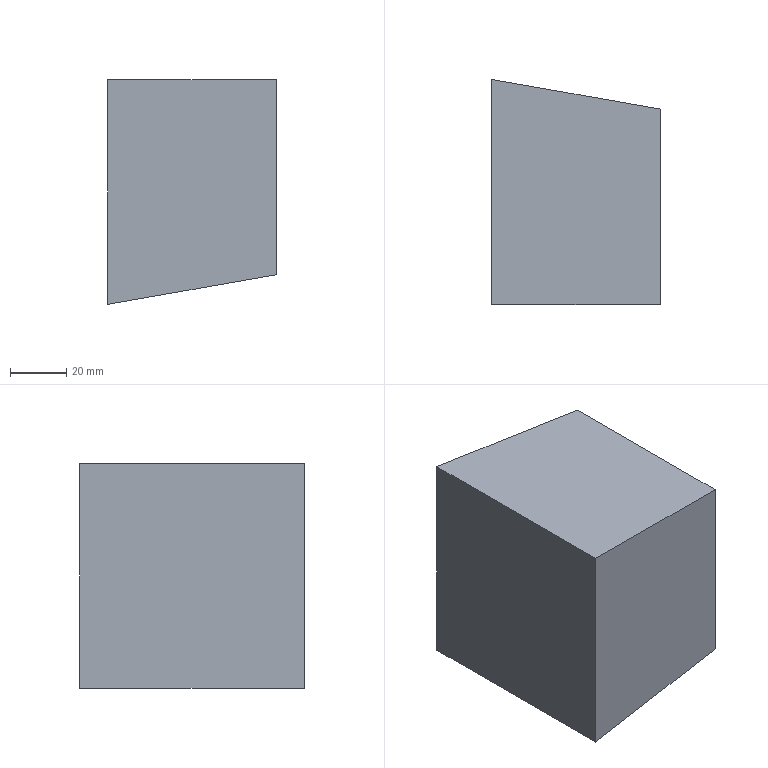Part | STEP file | solid 278 | 1 solid | 6 faces | box 60 x 80 x 80 mm | volume 335456 mm3 | plane 6